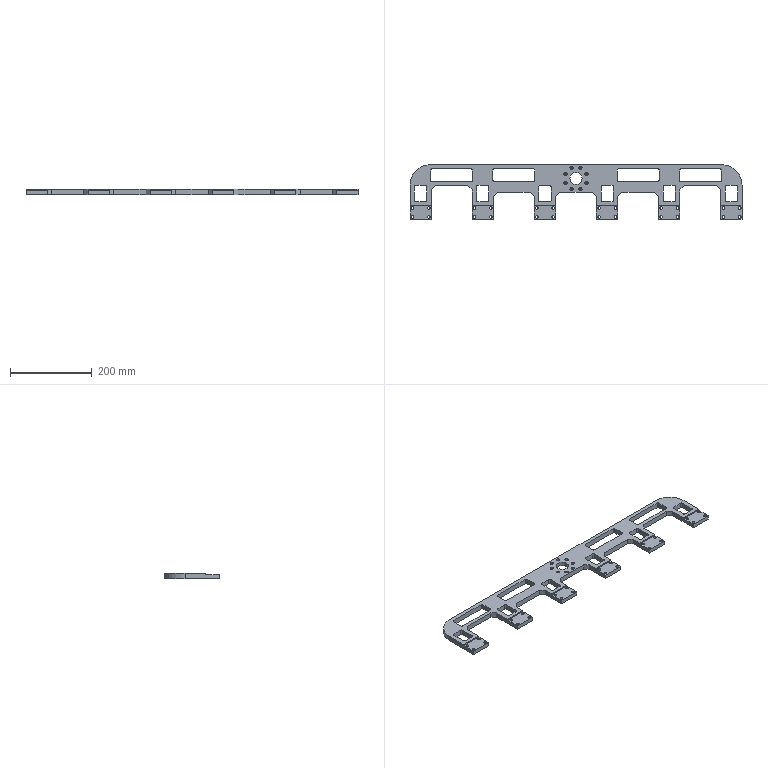NC program | NX | posted with a generic post | part box 813.6 x 134 x 13 mm
Lines 6266 to 7279 of 13853:
(HOLE_MILLING_COPY , TOOL : D6)
N12482 T06 M6
N12484 G54
N12486 G17 G0 G90 X-10.715 Y58.869 S9500 M3
N12488 G43 Z30. H6
N12490 Z0.5
N12492 G94 G3 X-10.215 Y58.369 R0.5 F1400.
N12494 X-9.715 Y58.869 R0.5
N12496 X-9.715 Y58.869 Z0. I-1. J0.
N12498 X-9.715 Y58.869 Z-0.5 I-1. J0.
N12500 X-9.715 Y58.869 Z-1. I-1. J0.
N12502 X-9.715 Y58.869 Z-1.5 I-1. J0.
N12504 X-9.715 Y58.869 Z-2. I-1. J0.
N12506 X-9.715 Y58.869 Z-2.5 I-1. J0.
N12508 X-9.715 Y58.869 Z-3. I-1. J0.
N12510 X-9.715 Y58.869 Z-3.5 I-1. J0.
N12512 X-9.715 Y58.869 Z-4. I-1. J0.
N12514 X-9.715 Y58.869 Z-4.5 I-1. J0.
N12516 X-10.406 Y59.82 Z-4.6 R1.
N12518 X-11.666 Y59.178 R1.
N12520 X-10.406 Y59.82 R-1.
N12522 X-11.036 Y59.499 R0.5
N12524 X-10.715 Y58.869 R0.5
N12526 G0 Z30.
N12528 X10.715
N12530 Z0.5
N12532 G3 X11.215 Y58.369 R0.5
N12534 X11.715 Y58.869 R0.5
N12536 X11.715 Y58.869 Z0. I-1. J0.
N12538 X11.715 Y58.869 Z-0.5 I-1. J0.
N12540 X11.715 Y58.869 Z-1. I-1. J0.
N12542 X11.715 Y58.869 Z-1.5 I-1. J0.
N12544 X11.715 Y58.869 Z-2. I-1. J0.
N12546 X11.715 Y58.869 Z-2.5 I-1. J0.
N12548 X11.715 Y58.869 Z-3. I-1. J0.
N12550 X11.715 Y58.869 Z-3.5 I-1. J0.
N12552 X11.715 Y58.869 Z-4. I-1. J0.
N12554 X11.715 Y58.869 Z-4.5 I-1. J0.
N12556 X11.024 Y59.82 Z-4.6 R1.
N12558 X9.764 Y59.178 R1.
N12560 X11.024 Y59.82 R-1.
N12562 X10.394 Y59.499 R0.5
N12564 X10.715 Y58.869 R0.5
N12566 G0 Z30.
N12568 X25.869 Y43.715
N12570 Z0.5
N12572 G3 X26.369 Y43.215 R0.5
N12574 X26.869 Y43.715 R0.5
N12576 X26.869 Y43.715 Z0. I-1. J0.
N12578 X26.869 Y43.715 Z-0.5 I-1. J0.
N12580 X26.869 Y43.715 Z-1. I-1. J0.
N12582 X26.869 Y43.715 Z-1.5 I-1. J0.
N12584 X26.869 Y43.715 Z-2. I-1. J0.
N12586 X26.869 Y43.715 Z-2.5 I-1. J0.
N12588 X26.869 Y43.715 Z-3. I-1. J0.
N12590 X26.869 Y43.715 Z-3.5 I-1. J0.
N12592 X26.869 Y43.715 Z-4. I-1. J0.
N12594 X26.869 Y43.715 Z-4.5 I-1. J0.
N12596 X26.178 Y44.666 Z-4.6 R1.
N12598 X24.918 Y44.024 R1.
N12600 X26.178 Y44.666 R-1.
N12602 X25.548 Y44.345 R0.5
N12604 X25.869 Y43.715 R0.5
N12606 G0 Z30.
N12608 Y22.285
N12610 Z0.5
N12612 G3 X26.369 Y21.785 R0.5
N12614 X26.869 Y22.285 R0.5
N12616 X26.869 Y22.285 Z0. I-1. J0.
N12618 X26.869 Y22.285 Z-0.5 I-1. J0.
N12620 X26.869 Y22.285 Z-1. I-1. J0.
N12622 X26.869 Y22.285 Z-1.5 I-1. J0.
N12624 X26.869 Y22.285 Z-2. I-1. J0.
N12626 X26.869 Y22.285 Z-2.5 I-1. J0.
N12628 X26.869 Y22.285 Z-3. I-1. J0.
N12630 X26.869 Y22.285 Z-3.5 I-1. J0.
N12632 X26.869 Y22.285 Z-4. I-1. J0.
N12634 X26.869 Y22.285 Z-4.5 I-1. J0.
N12636 X26.178 Y23.236 Z-4.6 R1.
N12638 X24.918 Y22.594 R1.
N12640 X26.178 Y23.236 R-1.
N12642 X25.548 Y22.915 R0.5
N12644 X25.869 Y22.285 R0.5
N12646 G0 Z30.
N12648 X10.715 Y7.131
N12650 Z0.5
N12652 G3 X11.215 Y6.631 R0.5
N12654 X11.715 Y7.131 R0.5
N12656 X11.715 Y7.131 Z0. I-1. J0.
N12658 X11.715 Y7.131 Z-0.5 I-1. J0.
N12660 X11.715 Y7.131 Z-1. I-1. J0.
N12662 X11.715 Y7.131 Z-1.5 I-1. J0.
N12664 X11.715 Y7.131 Z-2. I-1. J0.
N12666 X11.715 Y7.131 Z-2.5 I-1. J0.
N12668 X11.715 Y7.131 Z-3. I-1. J0.
N12670 X11.715 Y7.131 Z-3.5 I-1. J0.
N12672 X11.715 Y7.131 Z-4. I-1. J0.
N12674 X11.715 Y7.131 Z-4.5 I-1. J0.
N12676 X11.024 Y8.082 Z-4.6 R1.
N12678 X9.764 Y7.44 R1.
N12680 X11.024 Y8.082 R-1.
N12682 X10.394 Y7.761 R0.5
N12684 X10.715 Y7.131 R0.5
N12686 G0 Z30.
N12688 X-10.715
N12690 Z0.5
N12692 G3 X-10.215 Y6.631 R0.5
N12694 X-9.715 Y7.131 R0.5
N12696 X-9.715 Y7.131 Z0. I-1. J0.
N12698 X-9.715 Y7.131 Z-0.5 I-1. J0.
N12700 X-9.715 Y7.131 Z-1. I-1. J0.
N12702 X-9.715 Y7.131 Z-1.5 I-1. J0.
N12704 X-9.715 Y7.131 Z-2. I-1. J0.
N12706 X-9.715 Y7.131 Z-2.5 I-1. J0.
N12708 X-9.715 Y7.131 Z-3. I-1. J0.
N12710 X-9.715 Y7.131 Z-3.5 I-1. J0.
N12712 X-9.715 Y7.131 Z-4. I-1. J0.
N12714 X-9.715 Y7.131 Z-4.5 I-1. J0.
N12716 X-10.406 Y8.082 Z-4.6 R1.
N12718 X-11.666 Y7.44 R1.
N12720 X-10.406 Y8.082 R-1.
N12722 X-11.036 Y7.761 R0.5
N12724 X-10.715 Y7.131 R0.5
N12726 G0 Z30.
N12728 X-25.869 Y22.285
N12730 Z0.5
N12732 G3 X-25.369 Y21.785 R0.5
N12734 X-24.869 Y22.285 R0.5
N12736 X-24.869 Y22.285 Z0. I-1. J0.
N12738 X-24.869 Y22.285 Z-0.5 I-1. J0.
N12740 X-24.869 Y22.285 Z-1. I-1. J0.
N12742 X-24.869 Y22.285 Z-1.5 I-1. J0.
N12744 X-24.869 Y22.285 Z-2. I-1. J0.
N12746 X-24.869 Y22.285 Z-2.5 I-1. J0.
N12748 X-24.869 Y22.285 Z-3. I-1. J0.
N12750 X-24.869 Y22.285 Z-3.5 I-1. J0.
N12752 X-24.869 Y22.285 Z-4. I-1. J0.
N12754 X-24.869 Y22.285 Z-4.5 I-1. J0.
N12756 X-25.56 Y23.236 Z-4.6 R1.
N12758 X-26.82 Y22.594 R1.
N12760 X-25.56 Y23.236 R-1.
N12762 X-26.19 Y22.915 R0.5
N12764 X-25.869 Y22.285 R0.5
N12766 G0 Z30.
N12768 Y43.715
N12770 Z0.5
N12772 G3 X-25.369 Y43.215 R0.5
N12774 X-24.869 Y43.715 R0.5
N12776 X-24.869 Y43.715 Z0. I-1. J0.
N12778 X-24.869 Y43.715 Z-0.5 I-1. J0.
N12780 X-24.869 Y43.715 Z-1. I-1. J0.
N12782 X-24.869 Y43.715 Z-1.5 I-1. J0.
N12784 X-24.869 Y43.715 Z-2. I-1. J0.
N12786 X-24.869 Y43.715 Z-2.5 I-1. J0.
N12788 X-24.869 Y43.715 Z-3. I-1. J0.
N12790 X-24.869 Y43.715 Z-3.5 I-1. J0.
N12792 X-24.869 Y43.715 Z-4. I-1. J0.
N12794 X-24.869 Y43.715 Z-4.5 I-1. J0.
N12796 X-25.56 Y44.666 Z-4.6 R1.
N12798 X-26.82 Y44.024 R1.
N12800 X-25.56 Y44.666 R-1.
N12802 X-26.19 Y44.345 R0.5
N12804 X-25.869 Y43.715 R0.5
N12806 G0 Z30.
(ZLEVEL_PROFILE_COPY_1_COPY , TOOL : D6)
N12808 X-106.679 Y29.2
N12810 Z-0.591
N12812 G1 Y28.003 F1000.
N12814 X-106.616 Y28.
N12816 X-104.4 F1650.
N12818 Y30.216
N12820 X-104.403 Y30.279
N12822 X-105.6
N12824 G0 X-106.679 Y29.2 Z-1.182
N12826 G1 Y28.003 F1000.
N12828 X-106.616 Y28.
N12830 X-104.4 F1650.
N12832 Y30.216
N12834 X-104.403 Y30.279
N12836 X-105.6
N12838 G0 X-106.679 Y29.2 Z-1.773
N12840 G1 Y28.003 F1000.
N12842 X-106.616 Y28.
N12844 X-104.4 F1650.
N12846 Y30.216
N12848 X-104.403 Y30.279
N12850 X-105.6
N12852 G0 X-106.679 Y29.2 Z-2.364
N12854 G1 Y28.003 F1000.
N12856 X-106.616 Y28.
N12858 X-104.4 F1650.
N12860 Y30.216
N12862 X-104.403 Y30.279
N12864 X-105.6
N12866 G0 X-106.679 Y29.2 Z-2.955
N12868 G1 Y28.003 F1000.
N12870 X-106.616 Y28.
N12872 X-104.4 F1650.
N12874 Y30.216
N12876 X-104.403 Y30.279
N12878 X-105.6
N12880 G0 X-106.679 Y29.2 Z-3.545
N12882 G1 Y28.003 F1000.
N12884 X-106.616 Y28.
N12886 X-104.4 F1650.
N12888 Y30.216
N12890 X-104.403 Y30.279
N12892 X-105.6
N12894 G0 X-106.679 Y29.2 Z-4.136
N12896 G1 Y28.003 F1000.
N12898 X-106.616 Y28.
N12900 X-104.4 F1650.
N12902 Y30.216
N12904 X-104.403 Y30.279
N12906 X-105.6
N12908 G0 X-106.679 Y29.2 Z-4.727
N12910 G1 Y28.003 F1000.
N12912 X-106.616 Y28.
N12914 X-104.4 F1650.
N12916 Y30.216
N12918 X-104.403 Y30.279
N12920 X-105.6
N12922 G0 X-106.679 Y29.2 Z-5.318
N12924 G1 Y28.003 F1000.
N12926 X-106.616 Y28.
N12928 X-104.4 F1650.
N12930 Y30.216
N12932 X-104.403 Y30.279
N12934 X-105.6
N12936 G0 X-106.679 Y29.2 Z-5.909
N12938 G1 Y28.003 F1000.
N12940 X-106.616 Y28.
N12942 X-104.4 F1650.
N12944 Y30.216
N12946 X-104.403 Y30.279
N12948 X-105.6
N12950 G0 X-106.679 Y29.2 Z-6.5
N12952 G1 Y28.003 F1000.
N12954 X-106.616 Y28.
N12956 X-104.4 F1650.
N12958 Y30.216
N12960 X-104.403 Y30.279
N12962 X-105.6
N12964 G0 X-106.679 Y29.2 Z-7.091
N12966 G1 Y28.003 F1000.
N12968 X-106.616 Y28.
N12970 X-104.4 F1650.
N12972 Y30.216
N12974 X-104.403 Y30.279
N12976 X-105.6
N12978 G0 X-106.679 Y29.2 Z-7.682
N12980 G1 Y28.003 F1000.
N12982 X-106.616 Y28.
N12984 X-104.4 F1650.
N12986 Y30.216
N12988 X-104.403 Y30.279
N12990 X-105.6
N12992 G0 X-106.678 Y29.2 Z-8.273
N12994 G1 Y28.003 F1000.
N12996 X-106.615 Y28.
N12998 X-104.4 F1650.
N13000 Y30.209
N13002 X-104.403 Y30.272
N13004 X-105.6
N13006 G0 X-106.678 Y29.2 Z-8.864
N13008 G1 Y28.003 F1000.
N13010 X-106.615 Y28.
N13012 X-104.4 F1650.
N13014 Y30.209
N13016 X-104.403 Y30.272
N13018 X-105.6
N13020 G0 X-106.678 Y29.2 Z-9.455
N13022 G1 Y28.003 F1000.
N13024 X-106.615 Y28.
N13026 X-104.4 F1650.
N13028 Y30.209
N13030 X-104.403 Y30.272
N13032 X-105.6
N13034 G0 X-106.678 Y29.2 Z-10.045
N13036 G1 Y28.003 F1000.
N13038 X-106.615 Y28.
N13040 X-104.4 F1650.
N13042 Y30.209
N13044 X-104.403 Y30.272
N13046 X-105.6
N13048 G0 X-106.678 Y29.2 Z-10.636
N13050 G1 Y28.003 F1000.
N13052 X-106.615 Y28.
N13054 X-104.4 F1650.
N13056 Y30.209
N13058 X-104.403 Y30.272
N13060 X-105.6
N13062 G0 X-106.678 Y29.2 Z-11.227
N13064 G1 Y28.003 F1000.
N13066 X-106.615 Y28.
N13068 X-104.4 F1650.
N13070 Y30.209
N13072 X-104.403 Y30.272
N13074 X-105.6
N13076 G0 X-106.678 Y29.2 Z-11.818
N13078 G1 Y28.003 F1000.
N13080 X-106.615 Y28.
N13082 X-104.4 F1650.
N13084 Y30.209
N13086 X-104.403 Y30.272
N13088 X-105.6
N13090 G0 X-106.678 Y29.2 Z-12.409
N13092 G1 Y28.003 F1000.
N13094 X-106.615 Y28.
N13096 X-104.4 F1650.
N13098 Y30.209
N13100 X-104.403 Y30.272
N13102 X-105.6
N13104 G0 X-106.678 Y29.2 Z-13.
N13106 G1 Y28.003 F1000.
N13108 X-106.615 Y28.
N13110 X-104.4 F1650.
N13112 Y30.209
N13114 X-104.403 Y30.272
N13116 X-105.6
N13118 G0 Z30.
N13120 Y51.721
N13122 Z-0.591
N13124 G1 X-104.403 F1000.
N13126 X-104.4 Y51.784
N13128 Y54. F1650.
N13130 X-106.616
N13132 X-106.679 Y53.997
N13134 Y52.8
N13136 G0 X-105.6 Y51.721 Z-1.182
N13138 G1 X-104.403 F1000.
N13140 X-104.4 Y51.784
N13142 Y54. F1650.
N13144 X-106.616
N13146 X-106.679 Y53.997
N13148 Y52.8
N13150 G0 X-105.6 Y51.721 Z-1.773
N13152 G1 X-104.403 F1000.
N13154 X-104.4 Y51.784
N13156 Y54. F1650.
N13158 X-106.616
N13160 X-106.679 Y53.997
N13162 Y52.8
N13164 G0 X-105.6 Y51.721 Z-2.364
N13166 G1 X-104.403 F1000.
N13168 X-104.4 Y51.784
N13170 Y54. F1650.
N13172 X-106.616
N13174 X-106.679 Y53.997
N13176 Y52.8
N13178 G0 X-105.6 Y51.721 Z-2.955
N13180 G1 X-104.403 F1000.
N13182 X-104.4 Y51.784
N13184 Y54. F1650.
N13186 X-106.616
N13188 X-106.679 Y53.997
N13190 Y52.8
N13192 G0 X-105.6 Y51.721 Z-3.545
N13194 G1 X-104.403 F1000.
N13196 X-104.4 Y51.784
N13198 Y54. F1650.
N13200 X-106.616
N13202 X-106.679 Y53.997
N13204 Y52.8
N13206 G0 X-105.6 Y51.721 Z-4.136
N13208 G1 X-104.403 F1000.
N13210 X-104.4 Y51.784
N13212 Y54. F1650.
N13214 X-106.616
N13216 X-106.679 Y53.997
N13218 Y52.8
N13220 G0 X-105.6 Y51.721 Z-4.727
N13222 G1 X-104.403 F1000.
N13224 X-104.4 Y51.784
N13226 Y54. F1650.
N13228 X-106.616
N13230 X-106.679 Y53.997
N13232 Y52.8
N13234 G0 X-105.6 Y51.721 Z-5.318
N13236 G1 X-104.403 F1000.
N13238 X-104.4 Y51.784
N13240 Y54. F1650.
N13242 X-106.616
N13244 X-106.679 Y53.997
N13246 Y52.8
N13248 G0 X-105.6 Y51.721 Z-5.909
N13250 G1 X-104.403 F1000.
N13252 X-104.4 Y51.784
N13254 Y54. F1650.
N13256 X-106.616
N13258 X-106.679 Y53.997
N13260 Y52.8
N13262 G0 X-105.6 Y51.721 Z-6.5
N13264 G1 X-104.403 F1000.
N13266 X-104.4 Y51.784
N13268 Y54. F1650.
N13270 X-106.616
N13272 X-106.679 Y53.997
N13274 Y52.8
N13276 G0 X-105.6 Y51.721 Z-7.091
N13278 G1 X-104.403 F1000.
N13280 X-104.4 Y51.784
N13282 Y54. F1650.
N13284 X-106.616
N13286 X-106.679 Y53.997
N13288 Y52.8
N13290 G0 X-105.6 Y51.721 Z-7.682
N13292 G1 X-104.403 F1000.
N13294 X-104.4 Y51.784
N13296 Y54. F1650.
N13298 X-106.616
N13300 X-106.679 Y53.997
N13302 Y52.8
N13304 G0 X-105.6 Y51.725 Z-8.273
N13306 G1 X-104.403 F1000.
N13308 X-104.4 Y51.788
N13310 Y53.988 F1650.
N13312 Y54.
N13314 X-106.61
N13316 X-106.673 Y53.997
N13318 Y52.8
N13320 G0 X-105.6 Y51.725 Z-8.864
N13322 G1 X-104.403 F1000.
N13324 X-104.4 Y51.788
N13326 Y53.988 F1650.
N13328 Y54.
N13330 X-106.61
N13332 X-106.673 Y53.997
N13334 Y52.8
N13336 G0 X-105.6 Y51.725 Z-9.455
N13338 G1 X-104.403 F1000.
N13340 X-104.4 Y51.788
N13342 Y53.988 F1650.
N13344 Y54.
N13346 X-106.61
N13348 X-106.673 Y53.997
N13350 Y52.8
N13352 G0 X-105.6 Y51.725 Z-10.045
N13354 G1 X-104.403 F1000.
N13356 X-104.4 Y51.788
N13358 Y53.988 F1650.
N13360 Y54.
N13362 X-106.61
N13364 X-106.673 Y53.997
N13366 Y52.8
N13368 G0 X-105.6 Y51.725 Z-10.636
N13370 G1 X-104.403 F1000.
N13372 X-104.4 Y51.788
N13374 Y53.988 F1650.
N13376 Y54.
N13378 X-106.61
N13380 X-106.673 Y53.997
N13382 Y52.8
N13384 G0 X-105.6 Y51.725 Z-11.227
N13386 G1 X-104.403 F1000.
N13388 X-104.4 Y51.788
N13390 Y53.988 F1650.
N13392 Y54.
N13394 X-106.61
N13396 X-106.673 Y53.997
N13398 Y52.8
N13400 G0 X-105.6 Y51.725 Z-11.818
N13402 G1 X-104.403 F1000.
N13404 X-104.4 Y51.788
N13406 Y53.988 F1650.
N13408 Y54.
N13410 X-106.61
N13412 X-106.673 Y53.997
N13414 Y52.8
N13416 G0 X-105.6 Y51.725 Z-12.409
N13418 G1 X-104.403 F1000.
N13420 X-104.4 Y51.788
N13422 Y53.988 F1650.
N13424 Y54.
N13426 X-106.61
N13428 X-106.673 Y53.997
N13430 Y52.8
N13432 G0 X-105.6 Y51.725 Z-13.
N13434 G1 X-104.403 F1000.
N13436 X-104.4 Y51.788
N13438 Y53.988 F1650.
N13440 Y54.
N13442 X-106.61
N13444 X-106.673 Y53.997
N13446 Y52.8
N13448 G0 Z30.
N13450 X-198.121
N13452 Z-0.591
N13454 G1 Y53.997 F1000.
N13456 X-198.184 Y54.
N13458 X-200.4 F1650.
N13460 Y51.784
N13462 X-200.397 Y51.721
N13464 X-199.2
N13466 G0 X-198.121 Y52.8 Z-1.182
N13468 G1 Y53.997 F1000.
N13470 X-198.184 Y54.
N13472 X-200.4 F1650.
N13474 Y51.784
N13476 X-200.397 Y51.721
N13478 X-199.2
N13480 G0 X-198.121 Y52.8 Z-1.773
N13482 G1 Y53.997 F1000.
N13484 X-198.184 Y54.
N13486 X-200.4 F1650.
N13488 Y51.784
N13490 X-200.397 Y51.721
N13492 X-199.2
N13494 G0 X-198.121 Y52.8 Z-2.364
N13496 G1 Y53.997 F1000.
N13498 X-198.184 Y54.
N13500 X-200.4 F1650.
N13502 Y51.784
N13504 X-200.397 Y51.721
N13506 X-199.2
N13508 G0 X-198.121 Y52.8 Z-2.955
N13510 G1 Y53.997 F1000.
N13512 X-198.184 Y54.
N13514 X-200.4 F1650.
N13516 Y51.784
N13518 X-200.397 Y51.721
N13520 X-199.2
N13522 G0 X-198.121 Y52.8 Z-3.545
N13524 G1 Y53.997 F1000.
N13526 X-198.184 Y54.
N13528 X-200.4 F1650.
N13530 Y51.784
N13532 X-200.397 Y51.721
N13534 X-199.2
N13536 G0 X-198.121 Y52.8 Z-4.136
N13538 G1 Y53.997 F1000.
N13540 X-198.184 Y54.
N13542 X-200.4 F1650.
N13544 Y51.784
N13546 X-200.397 Y51.721
N13548 X-199.2
N13550 G0 X-198.121 Y52.8 Z-4.727
N13552 G1 Y53.997 F1000.
N13554 X-198.184 Y54.
N13556 X-200.4 F1650.
N13558 Y51.784
N13560 X-200.397 Y51.721
N13562 X-199.2
N13564 G0 X-198.121 Y52.8 Z-5.318
N13566 G1 Y53.997 F1000.
N13568 X-198.184 Y54.
N13570 X-200.4 F1650.
N13572 Y51.784
N13574 X-200.397 Y51.721
N13576 X-199.2
N13578 G0 X-198.121 Y52.8 Z-5.909
N13580 G1 Y53.997 F1000.
N13582 X-198.184 Y54.
N13584 X-200.4 F1650.
N13586 Y51.784
N13588 X-200.397 Y51.721
N13590 X-199.2
N13592 G0 X-198.121 Y52.8 Z-6.5
N13594 G1 Y53.997 F1000.
N13596 X-198.184 Y54.
N13598 X-200.4 F1650.
N13600 Y51.784
N13602 X-200.397 Y51.721
N13604 X-199.2
N13606 G0 X-198.121 Y52.8 Z-7.091
N13608 G1 Y53.997 F1000.
N13610 X-198.184 Y54.
N13612 X-200.4 F1650.
N13614 Y51.784
N13616 X-200.397 Y51.721
N13618 X-199.2
N13620 G0 X-198.121 Y52.8 Z-7.682
N13622 G1 Y53.997 F1000.
N13624 X-198.184 Y54.
N13626 X-200.4 F1650.
N13628 Y51.784
N13630 X-200.397 Y51.721
N13632 X-199.2
N13634 G0 X-198.131 Y52.8 Z-8.273
N13636 G1 Y53.997 F1000.
N13638 X-198.193 Y54.
N13640 X-200.4 F1650.
N13642 Y51.785
N13644 X-200.397 Y51.722
N13646 X-199.2
N13648 G0 X-198.131 Y52.8 Z-8.864
N13650 G1 Y53.997 F1000.
N13652 X-198.193 Y54.
N13654 X-200.4 F1650.
N13656 Y51.785
N13658 X-200.397 Y51.722
N13660 X-199.2
N13662 G0 X-198.131 Y52.8 Z-9.455
N13664 G1 Y53.997 F1000.
N13666 X-198.193 Y54.
N13668 X-200.4 F1650.
N13670 Y51.785
N13672 X-200.397 Y51.722
N13674 X-199.2
N13676 G0 X-198.131 Y52.8 Z-10.045
N13678 G1 Y53.997 F1000.
N13680 X-198.193 Y54.
N13682 X-200.4 F1650.
N13684 Y51.785
N13686 X-200.397 Y51.722
N13688 X-199.2
N13690 G0 X-198.131 Y52.8 Z-10.636
N13692 G1 Y53.997 F1000.
N13694 X-198.193 Y54.
N13696 X-200.4 F1650.
N13698 Y51.785
N13700 X-200.397 Y51.722
N13702 X-199.2
N13704 G0 X-198.131 Y52.8 Z-11.227
N13706 G1 Y53.997 F1000.
N13708 X-198.193 Y54.
N13710 X-200.4 F1650.
N13712 Y51.785
N13714 X-200.397 Y51.722
N13716 X-199.2
N13718 G0 X-198.131 Y52.8 Z-11.818
N13720 G1 Y53.997 F1000.
N13722 X-198.193 Y54.
N13724 X-200.4 F1650.
N13726 Y51.785
N13728 X-200.397 Y51.722
N13730 X-199.2
N13732 G0 X-198.131 Y52.8 Z-12.409
N13734 G1 Y53.997 F1000.
N13736 X-198.193 Y54.
N13738 X-200.4 F1650.
N13740 Y51.785
N13742 X-200.397 Y51.722
N13744 X-199.2
N13746 G0 X-198.131 Y52.8 Z-13.
N13748 G1 Y53.997 F1000.
N13750 X-198.193 Y54.
N13752 X-200.4 F1650.
N13754 Y51.785
N13756 X-200.397 Y51.722
N13758 X-199.2
N13760 G0 Z30.
N13762 Y30.279
N13764 Z-0.591
N13766 G1 X-200.397 F1000.
N13768 X-200.4 Y30.216
N13770 Y28.053 F1650.
N13772 X-200.401 Y27.999
N13774 X-200.386 Y28.
N13776 X-198.184
N13778 X-198.121 Y28.003
N13780 Y29.2
N13782 G0 X-199.2 Y30.279 Z-1.182
N13784 G1 X-200.397 F1000.
N13786 X-200.4 Y30.216
N13788 Y28.053 F1650.
N13790 X-200.401 Y27.999
N13792 X-200.386 Y28.
N13794 X-198.184
N13796 X-198.121 Y28.003
N13798 Y29.2
N13800 G0 X-199.2 Y30.279 Z-1.773
N13802 G1 X-200.397 F1000.
N13804 X-200.4 Y30.216
N13806 Y28.053 F1650.
N13808 X-200.401 Y27.999
N13810 X-200.386 Y28.
N13812 X-198.184
N13814 X-198.121 Y28.003
N13816 Y29.2
N13818 G0 X-199.2 Y30.279 Z-2.364
N13820 G1 X-200.397 F1000.
N13822 X-200.4 Y30.216
N13824 Y28.053 F1650.
N13826 X-200.401 Y27.999
N13828 X-200.386 Y28.
N13830 X-198.184
N13832 X-198.121 Y28.003
N13834 Y29.2
N13836 G0 X-199.2 Y30.279 Z-2.955
N13838 G1 X-200.397 F1000.
N13840 X-200.4 Y30.216
N13842 Y28.053 F1650.
N13844 X-200.401 Y27.999
N13846 X-200.386 Y28.
N13848 X-198.184
N13850 X-198.121 Y28.003
N13852 Y29.2
N13854 G0 X-199.2 Y30.279 Z-3.545
N13856 G1 X-200.397 F1000.
N13858 X-200.4 Y30.216
N13860 Y28.053 F1650.
N13862 X-200.401 Y27.999
N13864 X-198.184 Y28.
N13866 X-198.121 Y28.003
N13868 Y29.2
N13870 G0 X-199.2 Y30.279 Z-4.136
N13872 G1 X-200.397 F1000.
N13874 X-200.4 Y30.216
N13876 Y28.053 F1650.
N13878 X-200.401 Y27.999
N13880 X-198.184 Y28.
N13882 X-198.121 Y28.003
N13884 Y29.2
N13886 G0 X-199.2 Y30.279 Z-4.727
N13888 G1 X-200.397 F1000.
N13890 X-200.4 Y30.216
N13892 Y28. F1650.
N13894 X-198.184
N13896 X-198.121 Y28.003
N13898 Y29.2
N13900 G0 X-199.2 Y30.279 Z-5.318
N13902 G1 X-200.397 F1000.
N13904 X-200.4 Y30.216
N13906 Y28. F1650.
N13908 X-198.184
N13910 X-198.121 Y28.003
N13912 Y29.2
N13914 G0 X-199.2 Y30.279 Z-5.909
N13916 G1 X-200.397 F1000.
N13918 X-200.4 Y30.216
N13920 Y28. F1650.
N13922 X-198.184
N13924 X-198.121 Y28.003
N13926 Y29.2
N13928 G0 X-199.2 Y30.279 Z-6.5
N13930 G1 X-200.397 F1000.
N13932 X-200.4 Y30.216
N13934 Y28. F1650.
N13936 X-198.184
N13938 X-198.121 Y28.003
N13940 Y29.2
N13942 G0 X-199.2 Y30.279 Z-7.091
N13944 G1 X-200.397 F1000.
N13946 X-200.4 Y30.216
N13948 Y28. F1650.
N13950 X-198.184
N13952 X-198.121 Y28.003
N13954 Y29.2
N13956 G0 X-199.2 Y30.279 Z-7.682
N13958 G1 X-200.397 F1000.
N13960 X-200.4 Y30.216
N13962 Y28. F1650.
N13964 X-198.184
N13966 X-198.121 Y28.003
N13968 Y29.2
N13970 G0 X-199.2 Y30.279 Z-8.273
N13972 G1 X-200.397 F1000.
N13974 X-200.4 Y30.216
N13976 Y28. F1650.
N13978 X-198.184
N13980 X-198.121 Y28.003
N13982 Y29.2
N13984 G0 X-199.2 Y30.279 Z-8.864
N13986 G1 X-200.397 F1000.
N13988 X-200.4 Y30.216
N13990 Y28. F1650.
N13992 X-198.184
N13994 X-198.121 Y28.003
N13996 Y29.2
N13998 G0 X-199.2 Y30.279 Z-9.455
N14000 G1 X-200.397 F1000.
N14002 X-200.4 Y30.216
N14004 Y28. F1650.
N14006 X-198.184
N14008 X-198.121 Y28.003
N14010 Y29.2
N14012 G0 X-199.2 Y30.279 Z-10.045
N14014 G1 X-200.397 F1000.
N14016 X-200.4 Y30.216
N14018 Y28. F1650.
N14020 X-198.184
N14022 X-198.121 Y28.003
N14024 Y29.2
N14026 G0 X-199.2 Y30.279 Z-10.636
N14028 G1 X-200.397 F1000.
N14030 X-200.4 Y30.216
N14032 Y28. F1650.
N14034 X-198.184
N14036 X-198.121 Y28.003
N14038 Y29.2
N14040 G0 X-199.2 Y30.279 Z-11.227
N14042 G1 X-200.397 F1000.
N14044 X-200.4 Y30.216
N14046 Y28. F1650.
N14048 X-198.184
N14050 X-198.121 Y28.003
N14052 Y29.2
N14054 G0 X-199.2 Y30.279 Z-11.818
N14056 G1 X-200.397 F1000.
N14058 X-200.4 Y30.216
N14060 Y28. F1650.
N14062 X-198.184
N14064 X-198.121 Y28.003
N14066 Y29.2
N14068 G0 X-199.2 Y30.279 Z-12.409
N14070 G1 X-200.397 F1000.
N14072 X-200.4 Y30.216
N14074 Y28. F1650.
N14076 X-198.184
N14078 X-198.121 Y28.003
N14080 Y29.2
N14082 G0 X-199.2 Y30.279 Z-13.
N14084 G1 X-200.397 F1000.
N14086 X-200.4 Y30.216
N14088 Y28. F1650.
N14090 X-198.184
N14092 X-198.121 Y28.003
N14094 Y29.2
N14096 G0 Z30.
N14098 X-259.079
N14100 Z-0.591
N14102 G1 Y28.003 F1000.
N14104 X-259.016 Y28.
N14106 X-256.8 F1650.
N14108 Y30.216
N14110 X-256.803 Y30.279
N14112 X-258.
N14114 G0 X-259.079 Y29.2 Z-1.182
N14116 G1 Y28.003 F1000.
N14118 X-259.016 Y28.
N14120 X-256.8 F1650.
N14122 Y30.216
N14124 X-256.803 Y30.279
N14126 X-258.
N14128 G0 X-259.079 Y29.2 Z-1.773
N14130 G1 Y28.003 F1000.
N14132 X-259.016 Y28.
N14134 X-256.8 F1650.
N14136 Y30.216
N14138 X-256.803 Y30.279
N14140 X-258.
N14142 G0 X-259.079 Y29.2 Z-2.364
N14144 G1 Y28.003 F1000.
N14146 X-259.016 Y28.
N14148 X-256.8 F1650.
N14150 Y30.216
N14152 X-256.803 Y30.279
N14154 X-258.
N14156 G0 X-259.079 Y29.2 Z-2.955
N14158 G1 Y28.003 F1000.
N14160 X-259.016 Y28.
N14162 X-256.8 F1650.
N14164 Y30.216
N14166 X-256.803 Y30.279
N14168 X-258.
N14170 G0 X-259.079 Y29.2 Z-3.545
N14172 G1 Y28.003 F1000.
N14174 X-259.016 Y28.
N14176 X-256.8 F1650.
N14178 Y30.216
N14180 X-256.803 Y30.279
N14182 X-258.
N14184 G0 X-259.079 Y29.2 Z-4.136
N14186 G1 Y28.003 F1000.
N14188 X-259.016 Y28.
N14190 X-256.8 F1650.
N14192 Y30.216
N14194 X-256.803 Y30.279
N14196 X-258.
N14198 G0 X-259.079 Y29.2 Z-4.727
N14200 G1 Y28.003 F1000.
N14202 X-259.016 Y28.
N14204 X-256.8 F1650.
N14206 Y30.216
N14208 X-256.803 Y30.279
N14210 X-258.
N14212 G0 X-259.079 Y29.2 Z-5.318
N14214 G1 Y28.003 F1000.
N14216 X-259.016 Y28.
N14218 X-256.8 F1650.
N14220 Y30.216
N14222 X-256.803 Y30.279
N14224 X-258.
N14226 G0 X-259.079 Y29.2 Z-5.909
N14228 G1 Y28.003 F1000.
N14230 X-259.016 Y28.
N14232 X-256.8 F1650.
N14234 Y30.216
N14236 X-256.803 Y30.279
N14238 X-258.
N14240 G0 X-259.079 Y29.2 Z-6.5
N14242 G1 Y28.003 F1000.
N14244 X-259.016 Y28.
N14246 X-256.8 F1650.
N14248 Y30.216
N14250 X-256.803 Y30.279
N14252 X-258.
N14254 G0 X-259.079 Y29.2 Z-7.091
N14256 G1 Y28.003 F1000.
N14258 X-259.016 Y28.
N14260 X-256.8 F1650.
N14262 Y30.216
N14264 X-256.803 Y30.279
N14266 X-258.
N14268 G0 X-259.079 Y29.2 Z-7.682
N14270 G1 Y28.003 F1000.
N14272 X-259.016 Y28.
N14274 X-256.8 F1650.
N14276 Y30.216
N14278 X-256.803 Y30.279
N14280 X-258.
N14282 G0 X-259.091 Y29.2 Z-8.273
N14284 G1 Y28.003 F1000.
N14286 X-259.029 Y28.
N14288 X-256.8 F1650.
N14290 Y30.218
N14292 X-256.803 Y30.281
N14294 X-258.
N14296 G0 X-259.091 Y29.2 Z-8.864
N14298 G1 Y28.003 F1000.
N14300 X-259.029 Y28.
N14302 X-256.8 F1650.
N14304 Y30.218
N14306 X-256.803 Y30.281
N14308 X-258.
N14310 G0 X-259.091 Y29.2 Z-9.455
N14312 G1 Y28.003 F1000.
N14314 X-259.029 Y28.
N14316 X-256.8 F1650.
N14318 Y30.218
N14320 X-256.803 Y30.281
N14322 X-258.
N14324 G0 X-259.091 Y29.2 Z-10.045
N14326 G1 Y28.003 F1000.
N14328 X-259.029 Y28.
N14330 X-256.8 F1650.
N14332 Y30.218
N14334 X-256.803 Y30.281
N14336 X-258.
N14338 G0 X-259.091 Y29.2 Z-10.636
N14340 G1 Y28.003 F1000.
N14342 X-259.029 Y28.
N14344 X-256.8 F1650.
N14346 Y30.218
N14348 X-256.803 Y30.281
N14350 X-258.
N14352 G0 X-259.091 Y29.2 Z-11.227
N14354 G1 Y28.003 F1000.
N14356 X-259.029 Y28.
N14358 X-256.8 F1650.
N14360 Y30.218
N14362 X-256.803 Y30.281
N14364 X-258.
N14366 G0 X-259.091 Y29.2 Z-11.818
N14368 G1 Y28.003 F1000.
N14370 X-259.029 Y28.
N14372 X-256.8 F1650.
N14374 Y30.218
N14376 X-256.803 Y30.281
N14378 X-258.
N14380 G0 X-259.091 Y29.2 Z-12.409
N14382 G1 Y28.003 F1000.
N14384 X-259.029 Y28.
N14386 X-256.8 F1650.
N14388 Y30.218
N14390 X-256.803 Y30.281
N14392 X-258.
N14394 G0 X-259.091 Y29.2 Z-13.
N14396 G1 Y28.003 F1000.
N14398 X-259.029 Y28.
N14400 X-256.8 F1650.
N14402 Y30.218
N14404 X-256.803 Y30.281
N14406 X-258.
N14408 G0 Z30.
N14410 Y51.721
N14412 Z-0.591
N14414 G1 X-256.803 F1000.
N14416 X-256.8 Y51.784
N14418 Y54. F1650.
N14420 X-259.016
N14422 X-259.079 Y53.997
N14424 Y52.8
N14426 G0 X-258. Y51.721 Z-1.182
N14428 G1 X-256.803 F1000.
N14430 X-256.8 Y51.784
N14432 Y54. F1650.
N14434 X-259.016
N14436 X-259.079 Y53.997
N14438 Y52.8
N14440 G0 X-258. Y51.721 Z-1.773
N14442 G1 X-256.803 F1000.
N14444 X-256.8 Y51.784
N14446 Y54. F1650.
N14448 X-259.016
N14450 X-259.079 Y53.997
N14452 Y52.8
N14454 G0 X-258. Y51.721 Z-2.364
N14456 G1 X-256.803 F1000.
N14458 X-256.8 Y51.784
N14460 Y54. F1650.
N14462 X-259.016
N14464 X-259.079 Y53.997
N14466 Y52.8
N14468 G0 X-258. Y51.721 Z-2.955
N14470 G1 X-256.803 F1000.
N14472 X-256.8 Y51.784
N14474 Y54. F1650.
N14476 X-259.016
N14478 X-259.079 Y53.997
N14480 Y52.8
N14482 G0 X-258. Y51.721 Z-3.545
N14484 G1 X-256.803 F1000.
N14486 X-256.8 Y51.784
N14488 Y54. F1650.
N14490 X-259.016
N14492 X-259.079 Y53.997
N14494 Y52.8
N14496 G0 X-258. Y51.721 Z-4.136